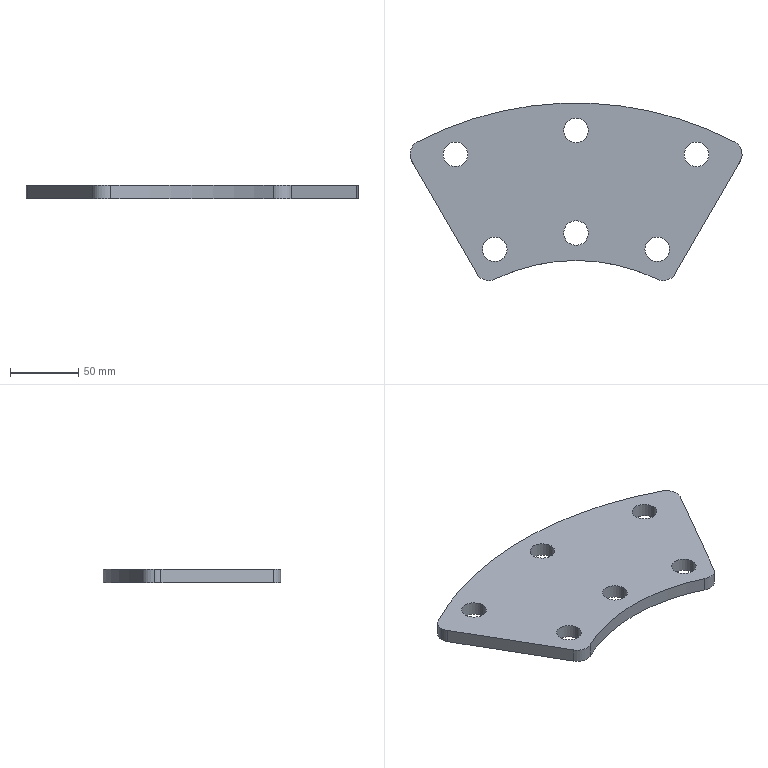Part | SolidWorks | features Extrusion 1, Fillet 1, ICE 1 | 1 solid | 23 faces | box 242.471 x 129.725 x 10 mm | volume 215713 mm3 | cylinder 19 | plane 4 | commonest cylinder face diameters 18 x12 20 x5 270 x1 500 x1
STEP:
#1=CARTESIAN_POINT('',(-97.017,212.492,0.));
#2=VERTEX_POINT('',#1);
#3=CARTESIAN_POINT('',(-79.017,212.492,0.));
#4=VERTEX_POINT('',#3);
#5=CARTESIAN_POINT('',(-88.017,212.492,0.));
#6=DIRECTION('',(0.,0.,1.));
#7=DIRECTION('',(-1.,0.,0.));
#8=AXIS2_PLACEMENT_3D('',#5,#6,#7);
#9=CIRCLE('',#8,9.);
#10=EDGE_CURVE('',#2,#4,#9,.T.);
#11=ORIENTED_EDGE('',*,*,#10,.F.);
#12=CARTESIAN_POINT('',(-97.017,212.492,10.));
#13=VERTEX_POINT('',#12);
#14=CARTESIAN_POINT('',(-97.017,212.492,0.));
#15=DIRECTION('',(0.,0.,1.));
#16=VECTOR('',#15,1000.);
#17=LINE('',#14,#16);
#18=EDGE_CURVE('',#2,#13,#17,.T.);
#19=ORIENTED_EDGE('',*,*,#18,.T.);
#20=CARTESIAN_POINT('',(-79.017,212.492,10.));
#21=VERTEX_POINT('',#20);
#22=CARTESIAN_POINT('',(-88.017,212.492,10.));
#23=DIRECTION('',(0.,0.,1.));
#24=DIRECTION('',(-1.,0.,0.));
#25=AXIS2_PLACEMENT_3D('',#22,#23,#24);
#26=CIRCLE('',#25,9.);
#27=EDGE_CURVE('',#13,#21,#26,.T.);
#28=ORIENTED_EDGE('',*,*,#27,.T.);
#29=CARTESIAN_POINT('',(-79.017,212.492,0.));
#30=DIRECTION('',(0.,0.,1.));
#31=VECTOR('',#30,1000.);
#32=LINE('',#29,#31);
#33=EDGE_CURVE('',#4,#21,#32,.T.);
#34=ORIENTED_EDGE('',*,*,#33,.F.);
#35=EDGE_LOOP('',(#11,#19,#28,#34));
#36=FACE_OUTER_BOUND('',#35,.T.);
#37=CARTESIAN_POINT('',(-88.017,212.492,0.));
#38=DIRECTION('',(0.,0.,1.));
#39=DIRECTION('',(1.,0.,0.));
#40=AXIS2_PLACEMENT_3D('',#37,#38,#39);
#41=CYLINDRICAL_SURFACE('',#40,9.);
#42=ADVANCED_FACE('',(#36),#41,.F.);
#43=CARTESIAN_POINT('',(79.017,212.492,0.));
#44=VERTEX_POINT('',#43);
#45=CARTESIAN_POINT('',(97.017,212.492,0.));
#46=VERTEX_POINT('',#45);
#47=CARTESIAN_POINT('',(88.017,212.492,0.));
#48=DIRECTION('',(0.,0.,1.));
#49=DIRECTION('',(1.,0.,0.));
#50=AXIS2_PLACEMENT_3D('',#47,#48,#49);
#51=CIRCLE('',#50,9.);
#52=EDGE_CURVE('',#44,#46,#51,.T.);
#53=ORIENTED_EDGE('',*,*,#52,.F.);
#54=CARTESIAN_POINT('',(79.017,212.492,10.));
#55=VERTEX_POINT('',#54);
#56=CARTESIAN_POINT('',(79.017,212.492,0.));
#57=DIRECTION('',(0.,0.,1.));
#58=VECTOR('',#57,1000.);
#59=LINE('',#56,#58);
#60=EDGE_CURVE('',#44,#55,#59,.T.);
#61=ORIENTED_EDGE('',*,*,#60,.T.);
#62=CARTESIAN_POINT('',(97.017,212.492,10.));
#63=VERTEX_POINT('',#62);
#64=CARTESIAN_POINT('',(88.017,212.492,10.));
#65=DIRECTION('',(0.,0.,1.));
#66=DIRECTION('',(1.,0.,0.));
#67=AXIS2_PLACEMENT_3D('',#64,#65,#66);
#68=CIRCLE('',#67,9.);
#69=EDGE_CURVE('',#55,#63,#68,.T.);
#70=ORIENTED_EDGE('',*,*,#69,.T.);
#71=CARTESIAN_POINT('',(97.017,212.492,0.));
#72=DIRECTION('',(0.,0.,1.));
#73=VECTOR('',#72,1000.);
#74=LINE('',#71,#73);
#75=EDGE_CURVE('',#46,#63,#74,.T.);
#76=ORIENTED_EDGE('',*,*,#75,.F.);
#77=EDGE_LOOP('',(#53,#61,#70,#76));
#78=FACE_OUTER_BOUND('',#77,.T.);
#79=CARTESIAN_POINT('',(88.017,212.492,0.));
#80=DIRECTION('',(0.,0.,1.));
#81=DIRECTION('',(1.,0.,0.));
#82=AXIS2_PLACEMENT_3D('',#79,#80,#81);
#83=CYLINDRICAL_SURFACE('',#82,9.);
#84=ADVANCED_FACE('',(#78),#83,.F.);
#85=CARTESIAN_POINT('',(-9.,230.,0.));
#86=VERTEX_POINT('',#85);
#87=CARTESIAN_POINT('',(9.,230.,0.));
#88=VERTEX_POINT('',#87);
#89=CARTESIAN_POINT('',(0.,230.,0.));
#90=DIRECTION('',(0.,0.,1.));
#91=DIRECTION('',(1.,0.,0.));
#92=AXIS2_PLACEMENT_3D('',#89,#90,#91);
#93=CIRCLE('',#92,9.);
#94=EDGE_CURVE('',#86,#88,#93,.T.);
#95=ORIENTED_EDGE('',*,*,#94,.F.);
#96=CARTESIAN_POINT('',(-9.,230.,10.));
#97=VERTEX_POINT('',#96);
#98=CARTESIAN_POINT('',(-9.,230.,0.));
#99=DIRECTION('',(0.,0.,1.));
#100=VECTOR('',#99,1000.);
#101=LINE('',#98,#100);
#102=EDGE_CURVE('',#86,#97,#101,.T.);
#103=ORIENTED_EDGE('',*,*,#102,.T.);
#104=CARTESIAN_POINT('',(9.,230.,10.));
#105=VERTEX_POINT('',#104);
#106=CARTESIAN_POINT('',(0.,230.,10.));
#107=DIRECTION('',(0.,0.,1.));
#108=DIRECTION('',(1.,0.,0.));
#109=AXIS2_PLACEMENT_3D('',#106,#107,#108);
#110=CIRCLE('',#109,9.);
#111=EDGE_CURVE('',#97,#105,#110,.T.);
#112=ORIENTED_EDGE('',*,*,#111,.T.);
#113=CARTESIAN_POINT('',(9.,230.,0.));
#114=DIRECTION('',(0.,0.,1.));
#115=VECTOR('',#114,1000.);
#116=LINE('',#113,#115);
#117=EDGE_CURVE('',#88,#105,#116,.T.);
#118=ORIENTED_EDGE('',*,*,#117,.F.);
#119=EDGE_LOOP('',(#95,#103,#112,#118));
#120=FACE_OUTER_BOUND('',#119,.T.);
#121=CARTESIAN_POINT('',(0.,230.,0.));
#122=DIRECTION('',(0.,0.,1.));
#123=DIRECTION('',(1.,0.,0.));
#124=AXIS2_PLACEMENT_3D('',#121,#122,#123);
#125=CYLINDRICAL_SURFACE('',#124,9.);
#126=ADVANCED_FACE('',(#120),#125,.F.);
#127=CARTESIAN_POINT('',(-121.236,212.666,10.));
#128=VERTEX_POINT('',#127);
#129=CARTESIAN_POINT('',(-119.896,207.666,10.));
#130=VERTEX_POINT('',#129);
#131=CARTESIAN_POINT('',(-111.236,212.666,10.));
#132=DIRECTION('',(0.,0.,1.));
#133=DIRECTION('',(1.,0.,0.));
#134=AXIS2_PLACEMENT_3D('',#131,#132,#133);
#135=CIRCLE('',#134,10.);
#136=EDGE_CURVE('',#128,#130,#135,.T.);
#137=ORIENTED_EDGE('',*,*,#136,.F.);
#138=CARTESIAN_POINT('',(-121.236,212.666,0.));
#139=VERTEX_POINT('',#138);
#140=CARTESIAN_POINT('',(-121.236,212.666,10.));
#141=DIRECTION('',(0.,0.,-1.));
#142=VECTOR('',#141,1000.);
#143=LINE('',#140,#142);
#144=EDGE_CURVE('',#128,#139,#143,.T.);
#145=ORIENTED_EDGE('',*,*,#144,.T.);
#146=CARTESIAN_POINT('',(-119.896,207.666,0.));
#147=VERTEX_POINT('',#146);
#148=CARTESIAN_POINT('',(-111.236,212.666,0.));
#149=DIRECTION('',(0.,0.,-1.));
#150=DIRECTION('',(1.,0.,0.));
#151=AXIS2_PLACEMENT_3D('',#148,#149,#150);
#152=CIRCLE('',#151,10.);
#153=EDGE_CURVE('',#147,#139,#152,.T.);
#154=ORIENTED_EDGE('',*,*,#153,.F.);
#155=CARTESIAN_POINT('',(-119.896,207.666,10.));
#156=DIRECTION('',(0.,0.,-1.));
#157=VECTOR('',#156,1000.);
#158=LINE('',#155,#157);
#159=EDGE_CURVE('',#130,#147,#158,.T.);
#160=ORIENTED_EDGE('',*,*,#159,.F.);
#161=EDGE_LOOP('',(#137,#145,#154,#160));
#162=FACE_OUTER_BOUND('',#161,.T.);
#163=CARTESIAN_POINT('',(-111.236,212.666,10.));
#164=DIRECTION('',(0.,0.,-1.));
#165=DIRECTION('',(-1.,0.,0.));
#166=AXIS2_PLACEMENT_3D('',#163,#164,#165);
#167=CYLINDRICAL_SURFACE('',#166,10.);
#168=ADVANCED_FACE('',(#162),#167,.T.);
#169=CARTESIAN_POINT('',(-68.316,143.201,10.));
#170=VERTEX_POINT('',#169);
#171=CARTESIAN_POINT('',(-50.316,143.201,10.));
#172=VERTEX_POINT('',#171);
#173=CARTESIAN_POINT('',(-59.316,143.201,10.));
#174=DIRECTION('',(0.,0.,1.));
#175=DIRECTION('',(1.,0.,0.));
#176=AXIS2_PLACEMENT_3D('',#173,#174,#175);
#177=CIRCLE('',#176,9.);
#178=EDGE_CURVE('',#170,#172,#177,.T.);
#179=ORIENTED_EDGE('',*,*,#178,.T.);
#180=CARTESIAN_POINT('',(-50.316,143.201,0.));
#181=VERTEX_POINT('',#180);
#182=CARTESIAN_POINT('',(-50.316,143.201,10.));
#183=DIRECTION('',(0.,0.,-1.));
#184=VECTOR('',#183,1000.);
#185=LINE('',#182,#184);
#186=EDGE_CURVE('',#172,#181,#185,.T.);
#187=ORIENTED_EDGE('',*,*,#186,.T.);
#188=CARTESIAN_POINT('',(-68.316,143.201,0.));
#189=VERTEX_POINT('',#188);
#190=CARTESIAN_POINT('',(-59.316,143.201,0.));
#191=DIRECTION('',(0.,0.,1.));
#192=DIRECTION('',(1.,0.,0.));
#193=AXIS2_PLACEMENT_3D('',#190,#191,#192);
#194=CIRCLE('',#193,9.);
#195=EDGE_CURVE('',#189,#181,#194,.T.);
#196=ORIENTED_EDGE('',*,*,#195,.F.);
#197=CARTESIAN_POINT('',(-68.316,143.201,10.));
#198=DIRECTION('',(0.,0.,-1.));
#199=VECTOR('',#198,1000.);
#200=LINE('',#197,#199);
#201=EDGE_CURVE('',#170,#189,#200,.T.);
#202=ORIENTED_EDGE('',*,*,#201,.F.);
#203=EDGE_LOOP('',(#179,#187,#196,#202));
#204=FACE_OUTER_BOUND('',#203,.T.);
#205=CARTESIAN_POINT('',(-59.316,143.201,10.));
#206=DIRECTION('',(0.,0.,-1.));
#207=DIRECTION('',(-1.,0.,0.));
#208=AXIS2_PLACEMENT_3D('',#205,#206,#207);
#209=CYLINDRICAL_SURFACE('',#208,9.);
#210=ADVANCED_FACE('',(#204),#209,.F.);
#211=CARTESIAN_POINT('',(50.316,143.201,10.));
#212=VERTEX_POINT('',#211);
#213=CARTESIAN_POINT('',(68.316,143.201,10.));
#214=VERTEX_POINT('',#213);
#215=CARTESIAN_POINT('',(59.316,143.201,10.));
#216=DIRECTION('',(0.,0.,1.));
#217=DIRECTION('',(1.,0.,0.));
#218=AXIS2_PLACEMENT_3D('',#215,#216,#217);
#219=CIRCLE('',#218,9.);
#220=EDGE_CURVE('',#212,#214,#219,.T.);
#221=ORIENTED_EDGE('',*,*,#220,.T.);
#222=CARTESIAN_POINT('',(68.316,143.201,0.));
#223=VERTEX_POINT('',#222);
#224=CARTESIAN_POINT('',(68.316,143.201,10.));
#225=DIRECTION('',(0.,0.,-1.));
#226=VECTOR('',#225,1000.);
#227=LINE('',#224,#226);
#228=EDGE_CURVE('',#214,#223,#227,.T.);
#229=ORIENTED_EDGE('',*,*,#228,.T.);
#230=CARTESIAN_POINT('',(50.316,143.201,0.));
#231=VERTEX_POINT('',#230);
#232=CARTESIAN_POINT('',(59.316,143.201,0.));
#233=DIRECTION('',(0.,0.,1.));
#234=DIRECTION('',(1.,0.,0.));
#235=AXIS2_PLACEMENT_3D('',#232,#233,#234);
#236=CIRCLE('',#235,9.);
#237=EDGE_CURVE('',#231,#223,#236,.T.);
#238=ORIENTED_EDGE('',*,*,#237,.F.);
#239=CARTESIAN_POINT('',(50.316,143.201,10.));
#240=DIRECTION('',(0.,0.,-1.));
#241=VECTOR('',#240,1000.);
#242=LINE('',#239,#241);
#243=EDGE_CURVE('',#212,#231,#242,.T.);
#244=ORIENTED_EDGE('',*,*,#243,.F.);
#245=EDGE_LOOP('',(#221,#229,#238,#244));
#246=FACE_OUTER_BOUND('',#245,.T.);
#247=CARTESIAN_POINT('',(59.316,143.201,10.));
#248=DIRECTION('',(0.,0.,-1.));
#249=DIRECTION('',(-1.,0.,0.));
#250=AXIS2_PLACEMENT_3D('',#247,#248,#249);
#251=CYLINDRICAL_SURFACE('',#250,9.);
#252=ADVANCED_FACE('',(#246),#251,.F.);
#253=CARTESIAN_POINT('',(-9.,155.,10.));
#254=VERTEX_POINT('',#253);
#255=CARTESIAN_POINT('',(9.,155.,10.));
#256=VERTEX_POINT('',#255);
#257=CARTESIAN_POINT('',(0.,155.,10.));
#258=DIRECTION('',(0.,0.,1.));
#259=DIRECTION('',(1.,0.,0.));
#260=AXIS2_PLACEMENT_3D('',#257,#258,#259);
#261=CIRCLE('',#260,9.);
#262=EDGE_CURVE('',#254,#256,#261,.T.);
#263=ORIENTED_EDGE('',*,*,#262,.T.);
#264=CARTESIAN_POINT('',(9.,155.,0.));
#265=VERTEX_POINT('',#264);
#266=CARTESIAN_POINT('',(9.,155.,10.));
#267=DIRECTION('',(0.,0.,-1.));
#268=VECTOR('',#267,1000.);
#269=LINE('',#266,#268);
#270=EDGE_CURVE('',#256,#265,#269,.T.);
#271=ORIENTED_EDGE('',*,*,#270,.T.);
#272=CARTESIAN_POINT('',(-9.,155.,0.));
#273=VERTEX_POINT('',#272);
#274=CARTESIAN_POINT('',(0.,155.,0.));
#275=DIRECTION('',(0.,0.,1.));
#276=DIRECTION('',(1.,0.,0.));
#277=AXIS2_PLACEMENT_3D('',#274,#275,#276);
#278=CIRCLE('',#277,9.);
#279=EDGE_CURVE('',#273,#265,#278,.T.);
#280=ORIENTED_EDGE('',*,*,#279,.F.);
#281=CARTESIAN_POINT('',(-9.,155.,10.));
#282=DIRECTION('',(0.,0.,-1.));
#283=VECTOR('',#282,1000.);
#284=LINE('',#281,#283);
#285=EDGE_CURVE('',#254,#273,#284,.T.);
#286=ORIENTED_EDGE('',*,*,#285,.F.);
#287=EDGE_LOOP('',(#263,#271,#280,#286));
#288=FACE_OUTER_BOUND('',#287,.T.);
#289=CARTESIAN_POINT('',(0.,155.,10.));
#290=DIRECTION('',(0.,0.,-1.));
#291=DIRECTION('',(-1.,0.,0.));
#292=AXIS2_PLACEMENT_3D('',#289,#290,#291);
#293=CYLINDRICAL_SURFACE('',#292,9.);
#294=ADVANCED_FACE('',(#288),#293,.F.);
#295=CARTESIAN_POINT('',(-88.017,212.492,10.));
#296=DIRECTION('',(0.,0.,1.));
#297=DIRECTION('',(-1.,0.,0.));
#298=AXIS2_PLACEMENT_3D('',#295,#296,#297);
#299=CIRCLE('',#298,9.);
#300=EDGE_CURVE('',#21,#13,#299,.T.);
#301=ORIENTED_EDGE('',*,*,#300,.F.);
#302=ORIENTED_EDGE('',*,*,#27,.F.);
#303=EDGE_LOOP('',(#301,#302));
#304=FACE_BOUND('',#303,.T.);
#305=CARTESIAN_POINT('',(88.017,212.492,10.));
#306=DIRECTION('',(0.,0.,1.));
#307=DIRECTION('',(1.,0.,0.));
#308=AXIS2_PLACEMENT_3D('',#305,#306,#307);
#309=CIRCLE('',#308,9.);
#310=EDGE_CURVE('',#63,#55,#309,.T.);
#311=ORIENTED_EDGE('',*,*,#310,.F.);
#312=ORIENTED_EDGE('',*,*,#69,.F.);
#313=EDGE_LOOP('',(#311,#312));
#314=FACE_BOUND('',#313,.T.);
#315=CARTESIAN_POINT('',(0.,230.,10.));
#316=DIRECTION('',(0.,0.,1.));
#317=DIRECTION('',(1.,0.,0.));
#318=AXIS2_PLACEMENT_3D('',#315,#316,#317);
#319=CIRCLE('',#318,9.);
#320=EDGE_CURVE('',#105,#97,#319,.T.);
#321=ORIENTED_EDGE('',*,*,#320,.F.);
#322=ORIENTED_EDGE('',*,*,#111,.F.);
#323=EDGE_LOOP('',(#321,#322));
#324=FACE_BOUND('',#323,.T.);
#325=ORIENTED_EDGE('',*,*,#220,.F.);
#326=CARTESIAN_POINT('',(59.316,143.201,10.));
#327=DIRECTION('',(0.,0.,1.));
#328=DIRECTION('',(1.,0.,0.));
#329=AXIS2_PLACEMENT_3D('',#326,#327,#328);
#330=CIRCLE('',#329,9.);
#331=EDGE_CURVE('',#214,#212,#330,.T.);
#332=ORIENTED_EDGE('',*,*,#331,.F.);
#333=EDGE_LOOP('',(#325,#332));
#334=FACE_BOUND('',#333,.T.);
#335=CARTESIAN_POINT('',(72.327,125.275,10.));
#336=VERTEX_POINT('',#335);
#337=CARTESIAN_POINT('',(119.896,207.666,10.));
#338=VERTEX_POINT('',#337);
#339=CARTESIAN_POINT('',(67.5,116.913,10.));
#340=DIRECTION('',(0.5,0.866,0.));
#341=VECTOR('',#340,1000.);
#342=LINE('',#339,#341);
#343=EDGE_CURVE('',#336,#338,#342,.T.);
#344=ORIENTED_EDGE('',*,*,#343,.T.);
#345=CARTESIAN_POINT('',(115.87,221.527,10.));
#346=VERTEX_POINT('',#345);
#347=CARTESIAN_POINT('',(111.236,212.666,10.));
#348=DIRECTION('',(0.,0.,1.));
#349=DIRECTION('',(1.,0.,0.));
#350=AXIS2_PLACEMENT_3D('',#347,#348,#349);
#351=CIRCLE('',#350,10.);
#352=EDGE_CURVE('',#338,#346,#351,.T.);
#353=ORIENTED_EDGE('',*,*,#352,.T.);
#354=CARTESIAN_POINT('',(-115.87,221.527,10.));
#355=VERTEX_POINT('',#354);
#356=CARTESIAN_POINT('',(0.,0.,10.));
#357=DIRECTION('',(0.,0.,1.));
#358=DIRECTION('',(1.,0.,0.));
#359=AXIS2_PLACEMENT_3D('',#356,#357,#358);
#360=CIRCLE('',#359,250.);
#361=EDGE_CURVE('',#346,#355,#360,.T.);
#362=ORIENTED_EDGE('',*,*,#361,.T.);
#363=CARTESIAN_POINT('',(-111.236,212.666,10.));
#364=DIRECTION('',(0.,0.,1.));
#365=DIRECTION('',(1.,0.,0.));
#366=AXIS2_PLACEMENT_3D('',#363,#364,#365);
#367=CIRCLE('',#366,10.);
#368=EDGE_CURVE('',#355,#128,#367,.T.);
#369=ORIENTED_EDGE('',*,*,#368,.T.);
#370=ORIENTED_EDGE('',*,*,#136,.T.);
#371=CARTESIAN_POINT('',(-72.327,125.275,10.));
#372=VERTEX_POINT('',#371);
#373=CARTESIAN_POINT('',(-67.5,116.913,10.));
#374=DIRECTION('',(0.5,-0.866,0.));
#375=VECTOR('',#374,1000.);
#376=LINE('',#373,#375);
#377=EDGE_CURVE('',#130,#372,#376,.T.);
#378=ORIENTED_EDGE('',*,*,#377,.T.);
#379=CARTESIAN_POINT('',(-59.276,121.29,10.));
#380=VERTEX_POINT('',#379);
#381=CARTESIAN_POINT('',(-63.667,130.275,10.));
#382=DIRECTION('',(0.,0.,1.));
#383=DIRECTION('',(1.,0.,0.));
#384=AXIS2_PLACEMENT_3D('',#381,#382,#383);
#385=CIRCLE('',#384,10.);
#386=EDGE_CURVE('',#372,#380,#385,.T.);
#387=ORIENTED_EDGE('',*,*,#386,.T.);
#388=CARTESIAN_POINT('',(59.276,121.29,10.));
#389=VERTEX_POINT('',#388);
#390=CARTESIAN_POINT('',(0.,0.,10.));
#391=DIRECTION('',(0.,0.,-1.));
#392=DIRECTION('',(1.,0.,0.));
#393=AXIS2_PLACEMENT_3D('',#390,#391,#392);
#394=CIRCLE('',#393,135.);
#395=EDGE_CURVE('',#380,#389,#394,.T.);
#396=ORIENTED_EDGE('',*,*,#395,.T.);
#397=CARTESIAN_POINT('',(63.667,130.275,10.));
#398=DIRECTION('',(0.,0.,1.));
#399=DIRECTION('',(1.,0.,0.));
#400=AXIS2_PLACEMENT_3D('',#397,#398,#399);
#401=CIRCLE('',#400,10.);
#402=EDGE_CURVE('',#389,#336,#401,.T.);
#403=ORIENTED_EDGE('',*,*,#402,.T.);
#404=EDGE_LOOP('',(#344,#353,#362,#369,#370,#378,#387,#396,#403));
#405=FACE_OUTER_BOUND('',#404,.T.);
#406=ORIENTED_EDGE('',*,*,#262,.F.);
#407=CARTESIAN_POINT('',(0.,155.,10.));
#408=DIRECTION('',(0.,0.,1.));
#409=DIRECTION('',(1.,0.,0.));
#410=AXIS2_PLACEMENT_3D('',#407,#408,#409);
#411=CIRCLE('',#410,9.);
#412=EDGE_CURVE('',#256,#254,#411,.T.);
#413=ORIENTED_EDGE('',*,*,#412,.F.);
#414=EDGE_LOOP('',(#406,#413));
#415=FACE_BOUND('',#414,.T.);
#416=ORIENTED_EDGE('',*,*,#178,.F.);
#417=CARTESIAN_POINT('',(-59.316,143.201,10.));
#418=DIRECTION('',(0.,0.,1.));
#419=DIRECTION('',(1.,0.,0.));
#420=AXIS2_PLACEMENT_3D('',#417,#418,#419);
#421=CIRCLE('',#420,9.);
#422=EDGE_CURVE('',#172,#170,#421,.T.);
#423=ORIENTED_EDGE('',*,*,#422,.F.);
#424=EDGE_LOOP('',(#416,#423));
#425=FACE_BOUND('',#424,.T.);
#426=CARTESIAN_POINT('',(0.,0.,10.));
#427=DIRECTION('',(0.,0.,1.));
#428=DIRECTION('',(1.,0.,0.));
#429=AXIS2_PLACEMENT_3D('',#426,#427,#428);
#430=PLANE('',#429);
#431=ADVANCED_FACE('',(#304,#314,#324,#334,#405,#415,#425),#430,.T.);
#432=CARTESIAN_POINT('',(-88.017,212.492,0.));
#433=DIRECTION('',(0.,0.,1.));
#434=DIRECTION('',(-1.,0.,0.));
#435=AXIS2_PLACEMENT_3D('',#432,#433,#434);
#436=CIRCLE('',#435,9.);
#437=EDGE_CURVE('',#4,#2,#436,.T.);
#438=ORIENTED_EDGE('',*,*,#437,.T.);
#439=ORIENTED_EDGE('',*,*,#10,.T.);
#440=EDGE_LOOP('',(#438,#439));
#441=FACE_BOUND('',#440,.T.);
#442=CARTESIAN_POINT('',(88.017,212.492,0.));
#443=DIRECTION('',(0.,0.,1.));
#444=DIRECTION('',(1.,0.,0.));
#445=AXIS2_PLACEMENT_3D('',#442,#443,#444);
#446=CIRCLE('',#445,9.);
#447=EDGE_CURVE('',#46,#44,#446,.T.);
#448=ORIENTED_EDGE('',*,*,#447,.T.);
#449=ORIENTED_EDGE('',*,*,#52,.T.);
#450=EDGE_LOOP('',(#448,#449));
#451=FACE_BOUND('',#450,.T.);
#452=CARTESIAN_POINT('',(0.,230.,0.));
#453=DIRECTION('',(0.,0.,1.));
#454=DIRECTION('',(1.,0.,0.));
#455=AXIS2_PLACEMENT_3D('',#452,#453,#454);
#456=CIRCLE('',#455,9.);
#457=EDGE_CURVE('',#88,#86,#456,.T.);
#458=ORIENTED_EDGE('',*,*,#457,.T.);
#459=ORIENTED_EDGE('',*,*,#94,.T.);
#460=EDGE_LOOP('',(#458,#459));
#461=FACE_BOUND('',#460,.T.);
#462=CARTESIAN_POINT('',(115.87,221.527,0.));
#463=VERTEX_POINT('',#462);
#464=CARTESIAN_POINT('',(-115.87,221.527,0.));
#465=VERTEX_POINT('',#464);
#466=CARTESIAN_POINT('',(0.,0.,0.));
#467=DIRECTION('',(0.,0.,1.));
#468=DIRECTION('',(1.,0.,0.));
#469=AXIS2_PLACEMENT_3D('',#466,#467,#468);
#470=CIRCLE('',#469,250.);
#471=EDGE_CURVE('',#463,#465,#470,.T.);
#472=ORIENTED_EDGE('',*,*,#471,.F.);
#473=CARTESIAN_POINT('',(119.896,207.666,0.));
#474=VERTEX_POINT('',#473);
#475=CARTESIAN_POINT('',(111.236,212.666,0.));
#476=DIRECTION('',(0.,0.,-1.));
#477=DIRECTION('',(1.,0.,0.));
#478=AXIS2_PLACEMENT_3D('',#475,#476,#477);
#479=CIRCLE('',#478,10.);
#480=EDGE_CURVE('',#463,#474,#479,.T.);
#481=ORIENTED_EDGE('',*,*,#480,.T.);
#482=CARTESIAN_POINT('',(72.327,125.275,0.));
#483=VERTEX_POINT('',#482);
#484=CARTESIAN_POINT('',(67.5,116.913,0.));
#485=DIRECTION('',(0.5,0.866,0.));
#486=VECTOR('',#485,1000.);
#487=LINE('',#484,#486);
#488=EDGE_CURVE('',#483,#474,#487,.T.);
#489=ORIENTED_EDGE('',*,*,#488,.F.);
#490=CARTESIAN_POINT('',(59.276,121.29,0.));
#491=VERTEX_POINT('',#490);
#492=CARTESIAN_POINT('',(63.667,130.275,0.));
#493=DIRECTION('',(0.,0.,-1.));
#494=DIRECTION('',(1.,0.,0.));
#495=AXIS2_PLACEMENT_3D('',#492,#493,#494);
#496=CIRCLE('',#495,10.);
#497=EDGE_CURVE('',#483,#491,#496,.T.);
#498=ORIENTED_EDGE('',*,*,#497,.T.);
#499=CARTESIAN_POINT('',(-59.276,121.29,0.));
#500=VERTEX_POINT('',#499);
#501=CARTESIAN_POINT('',(0.,0.,0.));
#502=DIRECTION('',(0.,0.,-1.));
#503=DIRECTION('',(1.,0.,0.));
#504=AXIS2_PLACEMENT_3D('',#501,#502,#503);
#505=CIRCLE('',#504,135.);
#506=EDGE_CURVE('',#500,#491,#505,.T.);
#507=ORIENTED_EDGE('',*,*,#506,.F.);
#508=CARTESIAN_POINT('',(-72.327,125.275,0.));
#509=VERTEX_POINT('',#508);
#510=CARTESIAN_POINT('',(-63.667,130.275,0.));
#511=DIRECTION('',(0.,0.,-1.));
#512=DIRECTION('',(1.,0.,0.));
#513=AXIS2_PLACEMENT_3D('',#510,#511,#512);
#514=CIRCLE('',#513,10.);
#515=EDGE_CURVE('',#500,#509,#514,.T.);
#516=ORIENTED_EDGE('',*,*,#515,.T.);
#517=CARTESIAN_POINT('',(-67.5,116.913,0.));
#518=DIRECTION('',(0.5,-0.866,0.));
#519=VECTOR('',#518,1000.);
#520=LINE('',#517,#519);
#521=EDGE_CURVE('',#147,#509,#520,.T.);
#522=ORIENTED_EDGE('',*,*,#521,.F.);
#523=ORIENTED_EDGE('',*,*,#153,.T.);
#524=CARTESIAN_POINT('',(-111.236,212.666,0.));
#525=DIRECTION('',(0.,0.,-1.));
#526=DIRECTION('',(1.,0.,0.));
#527=AXIS2_PLACEMENT_3D('',#524,#525,#526);
#528=CIRCLE('',#527,10.);
#529=EDGE_CURVE('',#139,#465,#528,.T.);
#530=ORIENTED_EDGE('',*,*,#529,.T.);
#531=EDGE_LOOP('',(#472,#481,#489,#498,#507,#516,#522,#523,#530));
#532=FACE_OUTER_BOUND('',#531,.T.);
#533=ORIENTED_EDGE('',*,*,#279,.T.);
#534=CARTESIAN_POINT('',(0.,155.,0.));
#535=DIRECTION('',(0.,0.,1.));
#536=DIRECTION('',(1.,0.,0.));
#537=AXIS2_PLACEMENT_3D('',#534,#535,#536);
#538=CIRCLE('',#537,9.);
#539=EDGE_CURVE('',#265,#273,#538,.T.);
#540=ORIENTED_EDGE('',*,*,#539,.T.);
#541=EDGE_LOOP('',(#533,#540));
#542=FACE_BOUND('',#541,.T.);
#543=ORIENTED_EDGE('',*,*,#237,.T.);
#544=CARTESIAN_POINT('',(59.316,143.201,0.));
#545=DIRECTION('',(0.,0.,1.));
#546=DIRECTION('',(1.,0.,0.));
#547=AXIS2_PLACEMENT_3D('',#544,#545,#546);
#548=CIRCLE('',#547,9.);
#549=EDGE_CURVE('',#223,#231,#548,.T.);
#550=ORIENTED_EDGE('',*,*,#549,.T.);
#551=EDGE_LOOP('',(#543,#550));
#552=FACE_BOUND('',#551,.T.);
#553=ORIENTED_EDGE('',*,*,#195,.T.);
#554=CARTESIAN_POINT('',(-59.316,143.201,0.));
#555=DIRECTION('',(0.,0.,1.));
#556=DIRECTION('',(1.,0.,0.));
#557=AXIS2_PLACEMENT_3D('',#554,#555,#556);
#558=CIRCLE('',#557,9.);
#559=EDGE_CURVE('',#181,#189,#558,.T.);
#560=ORIENTED_EDGE('',*,*,#559,.T.);
#561=EDGE_LOOP('',(#553,#560));
#562=FACE_BOUND('',#561,.T.);
#563=CARTESIAN_POINT('',(0.,0.,0.));
#564=DIRECTION('',(0.,0.,1.));
#565=DIRECTION('',(1.,0.,0.));
#566=AXIS2_PLACEMENT_3D('',#563,#564,#565);
#567=PLANE('',#566);
#568=ADVANCED_FACE('',(#441,#451,#461,#532,#542,#552,#562),#567,.F.);
#569=ORIENTED_EDGE('',*,*,#506,.T.);
#570=CARTESIAN_POINT('',(59.276,121.29,10.));
#571=DIRECTION('',(0.,0.,1.));
#572=VECTOR('',#571,1000.);
#573=LINE('',#570,#572);
#574=EDGE_CURVE('',#491,#389,#573,.T.);
#575=ORIENTED_EDGE('',*,*,#574,.T.);
#576=ORIENTED_EDGE('',*,*,#395,.F.);
#577=CARTESIAN_POINT('',(-59.276,121.29,10.));
#578=DIRECTION('',(0.,0.,-1.));
#579=VECTOR('',#578,1000.);
#580=LINE('',#577,#579);
#581=EDGE_CURVE('',#380,#500,#580,.T.);
#582=ORIENTED_EDGE('',*,*,#581,.T.);
#583=EDGE_LOOP('',(#569,#575,#576,#582));
#584=FACE_OUTER_BOUND('',#583,.T.);
#585=CARTESIAN_POINT('',(0.,0.,10.));
#586=DIRECTION('',(0.,0.,-1.));
#587=DIRECTION('',(-1.,0.,0.));
#588=AXIS2_PLACEMENT_3D('',#585,#586,#587);
#589=CYLINDRICAL_SURFACE('',#588,135.);
#590=ADVANCED_FACE('',(#584),#589,.F.);
#591=ORIENTED_EDGE('',*,*,#488,.T.);
#592=CARTESIAN_POINT('',(119.896,207.666,10.));
#593=DIRECTION('',(0.,0.,1.));
#594=VECTOR('',#593,1000.);
#595=LINE('',#592,#594);
#596=EDGE_CURVE('',#474,#338,#595,.T.);
#597=ORIENTED_EDGE('',*,*,#596,.T.);
#598=ORIENTED_EDGE('',*,*,#343,.F.);
#599=CARTESIAN_POINT('',(72.327,125.275,10.));
#600=DIRECTION('',(0.,0.,-1.));
#601=VECTOR('',#600,1000.);
#602=LINE('',#599,#601);
#603=EDGE_CURVE('',#336,#483,#602,.T.);
#604=ORIENTED_EDGE('',*,*,#603,.T.);
#605=EDGE_LOOP('',(#591,#597,#598,#604));
#606=FACE_OUTER_BOUND('',#605,.T.);
#607=CARTESIAN_POINT('',(67.5,116.913,10.));
#608=DIRECTION('',(-0.866,0.5,0.));
#609=DIRECTION('',(-0.5,-0.866,0.));
#610=AXIS2_PLACEMENT_3D('',#607,#608,#609);
#611=PLANE('',#610);
#612=ADVANCED_FACE('',(#606),#611,.F.);
#613=ORIENTED_EDGE('',*,*,#361,.F.);
#614=CARTESIAN_POINT('',(115.87,221.527,10.));
#615=DIRECTION('',(0.,0.,-1.));
#616=VECTOR('',#615,1000.);
#617=LINE('',#614,#616);
#618=EDGE_CURVE('',#346,#463,#617,.T.);
#619=ORIENTED_EDGE('',*,*,#618,.T.);
#620=ORIENTED_EDGE('',*,*,#471,.T.);
#621=CARTESIAN_POINT('',(-115.87,221.527,10.));
#622=DIRECTION('',(0.,0.,1.));
#623=VECTOR('',#622,1000.);
#624=LINE('',#621,#623);
#625=EDGE_CURVE('',#465,#355,#624,.T.);
#626=ORIENTED_EDGE('',*,*,#625,.T.);
#627=EDGE_LOOP('',(#613,#619,#620,#626));
#628=FACE_OUTER_BOUND('',#627,.T.);
#629=CARTESIAN_POINT('',(0.,0.,10.));
#630=DIRECTION('',(0.,0.,-1.));
#631=DIRECTION('',(-1.,0.,0.));
#632=AXIS2_PLACEMENT_3D('',#629,#630,#631);
#633=CYLINDRICAL_SURFACE('',#632,250.);
#634=ADVANCED_FACE('',(#628),#633,.T.);
#635=ORIENTED_EDGE('',*,*,#521,.T.);
#636=CARTESIAN_POINT('',(-72.327,125.275,10.));
#637=DIRECTION('',(0.,0.,1.));
#638=VECTOR('',#637,1000.);
#639=LINE('',#636,#638);
#640=EDGE_CURVE('',#509,#372,#639,.T.);
#641=ORIENTED_EDGE('',*,*,#640,.T.);
#642=ORIENTED_EDGE('',*,*,#377,.F.);
#643=ORIENTED_EDGE('',*,*,#159,.T.);
#644=EDGE_LOOP('',(#635,#641,#642,#643));
#645=FACE_OUTER_BOUND('',#644,.T.);
#646=CARTESIAN_POINT('',(-67.5,116.913,10.));
#647=DIRECTION('',(0.866,0.5,0.));
#648=DIRECTION('',(-0.5,0.866,0.));
#649=AXIS2_PLACEMENT_3D('',#646,#647,#648);
#650=PLANE('',#649);
#651=ADVANCED_FACE('',(#645),#650,.F.);
#652=ORIENTED_EDGE('',*,*,#270,.F.);
#653=ORIENTED_EDGE('',*,*,#412,.T.);
#654=ORIENTED_EDGE('',*,*,#285,.T.);
#655=ORIENTED_EDGE('',*,*,#539,.F.);
#656=EDGE_LOOP('',(#652,#653,#654,#655));
#657=FACE_OUTER_BOUND('',#656,.T.);
#658=CARTESIAN_POINT('',(0.,155.,10.));
#659=DIRECTION('',(0.,0.,-1.));
#660=DIRECTION('',(-1.,0.,0.));
#661=AXIS2_PLACEMENT_3D('',#658,#659,#660);
#662=CYLINDRICAL_SURFACE('',#661,9.);
#663=ADVANCED_FACE('',(#657),#662,.F.);
#664=ORIENTED_EDGE('',*,*,#228,.F.);
#665=ORIENTED_EDGE('',*,*,#331,.T.);
#666=ORIENTED_EDGE('',*,*,#243,.T.);
#667=ORIENTED_EDGE('',*,*,#549,.F.);
#668=EDGE_LOOP('',(#664,#665,#666,#667));
#669=FACE_OUTER_BOUND('',#668,.T.);
#670=CARTESIAN_POINT('',(59.316,143.201,10.));
#671=DIRECTION('',(0.,0.,-1.));
#672=DIRECTION('',(-1.,0.,0.));
#673=AXIS2_PLACEMENT_3D('',#670,#671,#672);
#674=CYLINDRICAL_SURFACE('',#673,9.);
#675=ADVANCED_FACE('',(#669),#674,.F.);
#676=ORIENTED_EDGE('',*,*,#186,.F.);
#677=ORIENTED_EDGE('',*,*,#422,.T.);
#678=ORIENTED_EDGE('',*,*,#201,.T.);
#679=ORIENTED_EDGE('',*,*,#559,.F.);
#680=EDGE_LOOP('',(#676,#677,#678,#679));
#681=FACE_OUTER_BOUND('',#680,.T.);
#682=CARTESIAN_POINT('',(-59.316,143.201,10.));
#683=DIRECTION('',(0.,0.,-1.));
#684=DIRECTION('',(-1.,0.,0.));
#685=AXIS2_PLACEMENT_3D('',#682,#683,#684);
#686=CYLINDRICAL_SURFACE('',#685,9.);
#687=ADVANCED_FACE('',(#681),#686,.F.);
#688=ORIENTED_EDGE('',*,*,#352,.F.);
#689=ORIENTED_EDGE('',*,*,#596,.F.);
#690=ORIENTED_EDGE('',*,*,#480,.F.);
#691=ORIENTED_EDGE('',*,*,#618,.F.);
#692=EDGE_LOOP('',(#688,#689,#690,#691));
#693=FACE_OUTER_BOUND('',#692,.T.);
#694=CARTESIAN_POINT('',(111.236,212.666,10.));
#695=DIRECTION('',(0.,0.,-1.));
#696=DIRECTION('',(-1.,0.,0.));
#697=AXIS2_PLACEMENT_3D('',#694,#695,#696);
#698=CYLINDRICAL_SURFACE('',#697,10.);
#699=ADVANCED_FACE('',(#693),#698,.T.);
#700=ORIENTED_EDGE('',*,*,#402,.F.);
#701=ORIENTED_EDGE('',*,*,#574,.F.);
#702=ORIENTED_EDGE('',*,*,#497,.F.);
#703=ORIENTED_EDGE('',*,*,#603,.F.);
#704=EDGE_LOOP('',(#700,#701,#702,#703));
#705=FACE_OUTER_BOUND('',#704,.T.);
#706=CARTESIAN_POINT('',(63.667,130.275,10.));
#707=DIRECTION('',(0.,0.,-1.));
#708=DIRECTION('',(-1.,0.,0.));
#709=AXIS2_PLACEMENT_3D('',#706,#707,#708);
#710=CYLINDRICAL_SURFACE('',#709,10.);
#711=ADVANCED_FACE('',(#705),#710,.T.);
#712=ORIENTED_EDGE('',*,*,#386,.F.);
#713=ORIENTED_EDGE('',*,*,#640,.F.);
#714=ORIENTED_EDGE('',*,*,#515,.F.);
#715=ORIENTED_EDGE('',*,*,#581,.F.);
#716=EDGE_LOOP('',(#712,#713,#714,#715));
#717=FACE_OUTER_BOUND('',#716,.T.);
#718=CARTESIAN_POINT('',(-63.667,130.275,10.));
#719=DIRECTION('',(0.,0.,-1.));
#720=DIRECTION('',(-1.,0.,0.));
#721=AXIS2_PLACEMENT_3D('',#718,#719,#720);
#722=CYLINDRICAL_SURFACE('',#721,10.);
#723=ADVANCED_FACE('',(#717),#722,.T.);
#724=ORIENTED_EDGE('',*,*,#144,.F.);
#725=ORIENTED_EDGE('',*,*,#368,.F.);
#726=ORIENTED_EDGE('',*,*,#625,.F.);
#727=ORIENTED_EDGE('',*,*,#529,.F.);
#728=EDGE_LOOP('',(#724,#725,#726,#727));
#729=FACE_OUTER_BOUND('',#728,.T.);
#730=CARTESIAN_POINT('',(-111.236,212.666,10.));
#731=DIRECTION('',(0.,0.,-1.));
#732=DIRECTION('',(-1.,0.,0.));
#733=AXIS2_PLACEMENT_3D('',#730,#731,#732);
#734=CYLINDRICAL_SURFACE('',#733,10.);
#735=ADVANCED_FACE('',(#729),#734,.T.);
#736=ORIENTED_EDGE('',*,*,#102,.F.);
#737=ORIENTED_EDGE('',*,*,#457,.F.);
#738=ORIENTED_EDGE('',*,*,#117,.T.);
#739=ORIENTED_EDGE('',*,*,#320,.T.);
#740=EDGE_LOOP('',(#736,#737,#738,#739));
#741=FACE_OUTER_BOUND('',#740,.T.);
#742=CARTESIAN_POINT('',(0.,230.,0.));
#743=DIRECTION('',(0.,0.,1.));
#744=DIRECTION('',(1.,0.,0.));
#745=AXIS2_PLACEMENT_3D('',#742,#743,#744);
#746=CYLINDRICAL_SURFACE('',#745,9.);
#747=ADVANCED_FACE('',(#741),#746,.F.);
#748=ORIENTED_EDGE('',*,*,#60,.F.);
#749=ORIENTED_EDGE('',*,*,#447,.F.);
#750=ORIENTED_EDGE('',*,*,#75,.T.);
#751=ORIENTED_EDGE('',*,*,#310,.T.);
#752=EDGE_LOOP('',(#748,#749,#750,#751));
#753=FACE_OUTER_BOUND('',#752,.T.);
#754=CARTESIAN_POINT('',(88.017,212.492,0.));
#755=DIRECTION('',(0.,0.,1.));
#756=DIRECTION('',(1.,0.,0.));
#757=AXIS2_PLACEMENT_3D('',#754,#755,#756);
#758=CYLINDRICAL_SURFACE('',#757,9.);
#759=ADVANCED_FACE('',(#753),#758,.F.);
#760=ORIENTED_EDGE('',*,*,#18,.F.);
#761=ORIENTED_EDGE('',*,*,#437,.F.);
#762=ORIENTED_EDGE('',*,*,#33,.T.);
#763=ORIENTED_EDGE('',*,*,#300,.T.);
#764=EDGE_LOOP('',(#760,#761,#762,#763));
#765=FACE_OUTER_BOUND('',#764,.T.);
#766=CARTESIAN_POINT('',(-88.017,212.492,0.));
#767=DIRECTION('',(0.,0.,1.));
#768=DIRECTION('',(1.,0.,0.));
#769=AXIS2_PLACEMENT_3D('',#766,#767,#768);
#770=CYLINDRICAL_SURFACE('',#769,9.);
#771=ADVANCED_FACE('',(#765),#770,.F.);
#772=CLOSED_SHELL('',(#42,#84,#126,#168,#210,#252,#294,#431,#568,#590,#612,#634,#651,#663,#675,#687,#699,#711,#723,#735,#747,#759,#771));
#773=MANIFOLD_SOLID_BREP('',#772);
#774=CARTESIAN_POINT('',(0.,0.,0.));
#775=DIRECTION('',(0.,0.,1.));
#776=DIRECTION('',(1.,0.,0.));
#777=AXIS2_PLACEMENT_3D('',#774,#775,#776);
#778=(LENGTH_UNIT()NAMED_UNIT(*)SI_UNIT(.MILLI.,.METRE.));
#779=UNCERTAINTY_MEASURE_WITH_UNIT(LENGTH_MEASURE(0.00001),#778,'','');
#780=(NAMED_UNIT(*)PLANE_ANGLE_UNIT()SI_UNIT($,.RADIAN.));
#781=(NAMED_UNIT(*)SI_UNIT($,.STERADIAN.)SOLID_ANGLE_UNIT());
#782=(GEOMETRIC_REPRESENTATION_CONTEXT(3)GLOBAL_UNCERTAINTY_ASSIGNED_CONTEXT((#779))GLOBAL_UNIT_ASSIGNED_CONTEXT((#778,#780,#781))REPRESENTATION_CONTEXT('',''));
#783=ADVANCED_BREP_SHAPE_REPRESENTATION('',(#773,#777),#782);